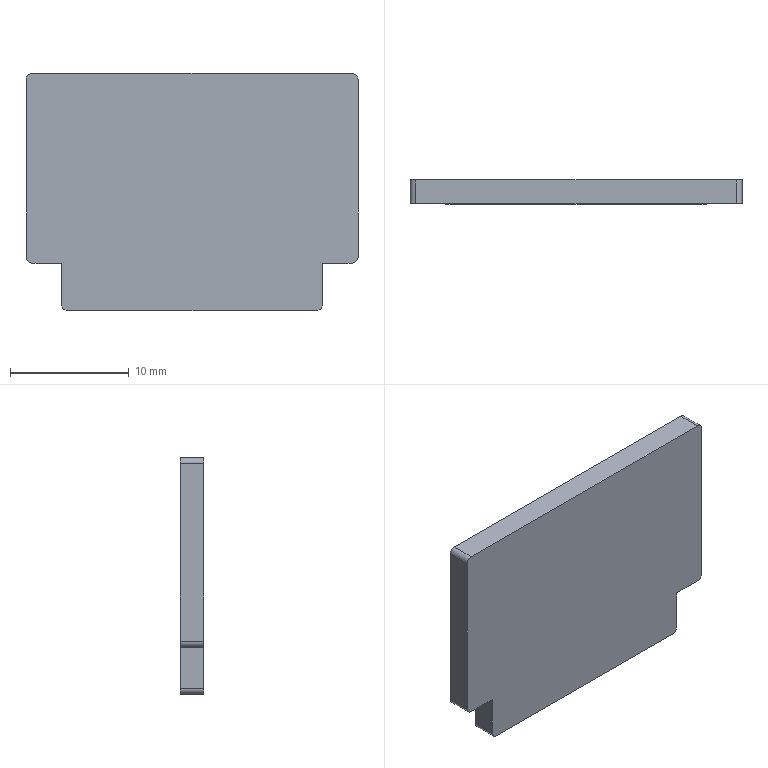Part | STEP file | Second C-100-B Work Part | 1 solid | 16 faces | box 28 x 2 x 20 mm | volume 1071 mm3 | plane 10 | cylinder 6 | commonest cylinder face diameters 1 x6
STEP:
#1=CARTESIAN_POINT('',(-11.,2.,-14.2));
#2=VERTEX_POINT('',#1);
#3=CARTESIAN_POINT('',(-10.5,2.,-14.7));
#4=VERTEX_POINT('',#3);
#5=CARTESIAN_POINT('',(-10.5,2.,-14.2));
#6=DIRECTION('',(0.,-1.,0.));
#7=DIRECTION('',(0.,0.,-1.));
#8=AXIS2_PLACEMENT_3D('',#5,#6,#7);
#9=CIRCLE('',#8,0.5);
#10=EDGE_CURVE('',#2,#4,#9,.T.);
#11=ORIENTED_EDGE('',*,*,#10,.F.);
#12=CARTESIAN_POINT('',(-11.,2.,-10.7));
#13=VERTEX_POINT('',#12);
#14=CARTESIAN_POINT('',(-11.,2.,-10.2));
#15=DIRECTION('',(0.,0.,1.));
#16=VECTOR('',#15,1000.);
#17=LINE('',#14,#16);
#18=EDGE_CURVE('',#2,#13,#17,.T.);
#19=ORIENTED_EDGE('',*,*,#18,.T.);
#20=CARTESIAN_POINT('',(-13.5,2.,-10.7));
#21=VERTEX_POINT('',#20);
#22=CARTESIAN_POINT('',(-13.5,2.,-10.7));
#23=DIRECTION('',(-1.,0.,0.));
#24=VECTOR('',#23,1000.);
#25=LINE('',#22,#24);
#26=EDGE_CURVE('',#13,#21,#25,.T.);
#27=ORIENTED_EDGE('',*,*,#26,.T.);
#28=CARTESIAN_POINT('',(-14.,2.,-10.2));
#29=VERTEX_POINT('',#28);
#30=CARTESIAN_POINT('',(-13.5,2.,-10.2));
#31=DIRECTION('',(0.,-1.,0.));
#32=DIRECTION('',(0.,0.,-1.));
#33=AXIS2_PLACEMENT_3D('',#30,#31,#32);
#34=CIRCLE('',#33,0.5);
#35=EDGE_CURVE('',#29,#21,#34,.T.);
#36=ORIENTED_EDGE('',*,*,#35,.F.);
#37=CARTESIAN_POINT('',(-14.,2.,4.8));
#38=VERTEX_POINT('',#37);
#39=CARTESIAN_POINT('',(-14.,2.,-10.2));
#40=DIRECTION('',(0.,0.,1.));
#41=VECTOR('',#40,1000.);
#42=LINE('',#39,#41);
#43=EDGE_CURVE('',#29,#38,#42,.T.);
#44=ORIENTED_EDGE('',*,*,#43,.T.);
#45=CARTESIAN_POINT('',(-13.5,2.,5.3));
#46=VERTEX_POINT('',#45);
#47=CARTESIAN_POINT('',(-13.5,2.,4.8));
#48=DIRECTION('',(0.,-1.,0.));
#49=DIRECTION('',(0.,0.,-1.));
#50=AXIS2_PLACEMENT_3D('',#47,#48,#49);
#51=CIRCLE('',#50,0.5);
#52=EDGE_CURVE('',#46,#38,#51,.T.);
#53=ORIENTED_EDGE('',*,*,#52,.F.);
#54=CARTESIAN_POINT('',(13.5,2.,5.3));
#55=VERTEX_POINT('',#54);
#56=CARTESIAN_POINT('',(-13.5,2.,5.3));
#57=DIRECTION('',(1.,0.,0.));
#58=VECTOR('',#57,1000.);
#59=LINE('',#56,#58);
#60=EDGE_CURVE('',#46,#55,#59,.T.);
#61=ORIENTED_EDGE('',*,*,#60,.T.);
#62=CARTESIAN_POINT('',(14.,2.,4.8));
#63=VERTEX_POINT('',#62);
#64=CARTESIAN_POINT('',(13.5,2.,4.8));
#65=DIRECTION('',(0.,-1.,0.));
#66=DIRECTION('',(0.,0.,-1.));
#67=AXIS2_PLACEMENT_3D('',#64,#65,#66);
#68=CIRCLE('',#67,0.5);
#69=EDGE_CURVE('',#63,#55,#68,.T.);
#70=ORIENTED_EDGE('',*,*,#69,.F.);
#71=CARTESIAN_POINT('',(14.,2.,-10.2));
#72=VERTEX_POINT('',#71);
#73=CARTESIAN_POINT('',(14.,2.,-10.2));
#74=DIRECTION('',(0.,0.,-1.));
#75=VECTOR('',#74,1000.);
#76=LINE('',#73,#75);
#77=EDGE_CURVE('',#63,#72,#76,.T.);
#78=ORIENTED_EDGE('',*,*,#77,.T.);
#79=CARTESIAN_POINT('',(13.5,2.,-10.7));
#80=VERTEX_POINT('',#79);
#81=CARTESIAN_POINT('',(13.5,2.,-10.2));
#82=DIRECTION('',(0.,-1.,0.));
#83=DIRECTION('',(0.,0.,-1.));
#84=AXIS2_PLACEMENT_3D('',#81,#82,#83);
#85=CIRCLE('',#84,0.5);
#86=EDGE_CURVE('',#80,#72,#85,.T.);
#87=ORIENTED_EDGE('',*,*,#86,.F.);
#88=CARTESIAN_POINT('',(11.,2.,-10.7));
#89=VERTEX_POINT('',#88);
#90=CARTESIAN_POINT('',(-13.5,2.,-10.7));
#91=DIRECTION('',(-1.,0.,0.));
#92=VECTOR('',#91,1000.);
#93=LINE('',#90,#92);
#94=EDGE_CURVE('',#80,#89,#93,.T.);
#95=ORIENTED_EDGE('',*,*,#94,.T.);
#96=CARTESIAN_POINT('',(11.,2.,-14.2));
#97=VERTEX_POINT('',#96);
#98=CARTESIAN_POINT('',(11.,2.,-10.2));
#99=DIRECTION('',(0.,0.,-1.));
#100=VECTOR('',#99,1000.);
#101=LINE('',#98,#100);
#102=EDGE_CURVE('',#89,#97,#101,.T.);
#103=ORIENTED_EDGE('',*,*,#102,.T.);
#104=CARTESIAN_POINT('',(10.5,2.,-14.7));
#105=VERTEX_POINT('',#104);
#106=CARTESIAN_POINT('',(10.5,2.,-14.2));
#107=DIRECTION('',(0.,-1.,0.));
#108=DIRECTION('',(0.,0.,-1.));
#109=AXIS2_PLACEMENT_3D('',#106,#107,#108);
#110=CIRCLE('',#109,0.5);
#111=EDGE_CURVE('',#105,#97,#110,.T.);
#112=ORIENTED_EDGE('',*,*,#111,.F.);
#113=CARTESIAN_POINT('',(-13.5,2.,-14.7));
#114=DIRECTION('',(-1.,0.,0.));
#115=VECTOR('',#114,1000.);
#116=LINE('',#113,#115);
#117=EDGE_CURVE('',#105,#4,#116,.T.);
#118=ORIENTED_EDGE('',*,*,#117,.T.);
#119=EDGE_LOOP('',(#11,#19,#27,#36,#44,#53,#61,#70,#78,#87,#95,#103,#112,#118));
#120=FACE_OUTER_BOUND('',#119,.T.);
#121=CARTESIAN_POINT('',(-13.5,2.,-10.2));
#122=DIRECTION('',(0.,1.,0.));
#123=DIRECTION('',(0.,0.,1.));
#124=AXIS2_PLACEMENT_3D('',#121,#122,#123);
#125=PLANE('',#124);
#126=ADVANCED_FACE('',(#120),#125,.T.);
#127=CARTESIAN_POINT('',(-11.,0.,-10.7));
#128=VERTEX_POINT('',#127);
#129=CARTESIAN_POINT('',(-11.,2.,-10.7));
#130=DIRECTION('',(0.,-1.,0.));
#131=VECTOR('',#130,1000.);
#132=LINE('',#129,#131);
#133=EDGE_CURVE('',#13,#128,#132,.T.);
#134=ORIENTED_EDGE('',*,*,#133,.F.);
#135=ORIENTED_EDGE('',*,*,#18,.F.);
#136=CARTESIAN_POINT('',(-11.,0.,-14.2));
#137=VERTEX_POINT('',#136);
#138=CARTESIAN_POINT('',(-11.,2.,-14.2));
#139=DIRECTION('',(0.,1.,0.));
#140=VECTOR('',#139,1000.);
#141=LINE('',#138,#140);
#142=EDGE_CURVE('',#137,#2,#141,.T.);
#143=ORIENTED_EDGE('',*,*,#142,.F.);
#144=CARTESIAN_POINT('',(-11.,0.,-10.7));
#145=DIRECTION('',(0.,0.,-1.));
#146=VECTOR('',#145,1000.);
#147=LINE('',#144,#146);
#148=EDGE_CURVE('',#128,#137,#147,.T.);
#149=ORIENTED_EDGE('',*,*,#148,.F.);
#150=EDGE_LOOP('',(#134,#135,#143,#149));
#151=FACE_OUTER_BOUND('',#150,.T.);
#152=CARTESIAN_POINT('',(-11.,2.,-10.7));
#153=DIRECTION('',(1.,0.,0.));
#154=DIRECTION('',(0.,0.,-1.));
#155=AXIS2_PLACEMENT_3D('',#152,#153,#154);
#156=PLANE('',#155);
#157=ADVANCED_FACE('',(#151),#156,.F.);
#158=CARTESIAN_POINT('',(-10.5,0.,-14.7));
#159=VERTEX_POINT('',#158);
#160=CARTESIAN_POINT('',(-10.5,2.,-14.7));
#161=DIRECTION('',(0.,-1.,0.));
#162=VECTOR('',#161,1000.);
#163=LINE('',#160,#162);
#164=EDGE_CURVE('',#4,#159,#163,.T.);
#165=ORIENTED_EDGE('',*,*,#164,.F.);
#166=ORIENTED_EDGE('',*,*,#117,.F.);
#167=CARTESIAN_POINT('',(10.5,0.,-14.7));
#168=VERTEX_POINT('',#167);
#169=CARTESIAN_POINT('',(10.5,2.,-14.7));
#170=DIRECTION('',(0.,1.,0.));
#171=VECTOR('',#170,1000.);
#172=LINE('',#169,#171);
#173=EDGE_CURVE('',#168,#105,#172,.T.);
#174=ORIENTED_EDGE('',*,*,#173,.F.);
#175=CARTESIAN_POINT('',(-10.5,0.,-14.7));
#176=DIRECTION('',(1.,0.,0.));
#177=VECTOR('',#176,1000.);
#178=LINE('',#175,#177);
#179=EDGE_CURVE('',#159,#168,#178,.T.);
#180=ORIENTED_EDGE('',*,*,#179,.F.);
#181=EDGE_LOOP('',(#165,#166,#174,#180));
#182=FACE_OUTER_BOUND('',#181,.T.);
#183=CARTESIAN_POINT('',(-10.5,2.,-14.7));
#184=DIRECTION('',(0.,0.,1.));
#185=DIRECTION('',(1.,0.,0.));
#186=AXIS2_PLACEMENT_3D('',#183,#184,#185);
#187=PLANE('',#186);
#188=ADVANCED_FACE('',(#182),#187,.F.);
#189=CARTESIAN_POINT('',(11.,0.,-14.2));
#190=VERTEX_POINT('',#189);
#191=CARTESIAN_POINT('',(11.,2.,-14.2));
#192=DIRECTION('',(0.,-1.,0.));
#193=VECTOR('',#192,1000.);
#194=LINE('',#191,#193);
#195=EDGE_CURVE('',#97,#190,#194,.T.);
#196=ORIENTED_EDGE('',*,*,#195,.F.);
#197=ORIENTED_EDGE('',*,*,#102,.F.);
#198=CARTESIAN_POINT('',(11.,0.,-10.7));
#199=VERTEX_POINT('',#198);
#200=CARTESIAN_POINT('',(11.,2.,-10.7));
#201=DIRECTION('',(0.,1.,0.));
#202=VECTOR('',#201,1000.);
#203=LINE('',#200,#202);
#204=EDGE_CURVE('',#199,#89,#203,.T.);
#205=ORIENTED_EDGE('',*,*,#204,.F.);
#206=CARTESIAN_POINT('',(11.,0.,-14.2));
#207=DIRECTION('',(0.,0.,1.));
#208=VECTOR('',#207,1000.);
#209=LINE('',#206,#208);
#210=EDGE_CURVE('',#190,#199,#209,.T.);
#211=ORIENTED_EDGE('',*,*,#210,.F.);
#212=EDGE_LOOP('',(#196,#197,#205,#211));
#213=FACE_OUTER_BOUND('',#212,.T.);
#214=CARTESIAN_POINT('',(11.,2.,-14.2));
#215=DIRECTION('',(-1.,0.,0.));
#216=DIRECTION('',(0.,0.,1.));
#217=AXIS2_PLACEMENT_3D('',#214,#215,#216);
#218=PLANE('',#217);
#219=ADVANCED_FACE('',(#213),#218,.F.);
#220=ORIENTED_EDGE('',*,*,#204,.T.);
#221=ORIENTED_EDGE('',*,*,#94,.F.);
#222=CARTESIAN_POINT('',(13.5,0.,-10.7));
#223=VERTEX_POINT('',#222);
#224=CARTESIAN_POINT('',(13.5,2.,-10.7));
#225=DIRECTION('',(0.,1.,0.));
#226=VECTOR('',#225,1000.);
#227=LINE('',#224,#226);
#228=EDGE_CURVE('',#223,#80,#227,.T.);
#229=ORIENTED_EDGE('',*,*,#228,.F.);
#230=CARTESIAN_POINT('',(13.5,0.,-10.7));
#231=DIRECTION('',(1.,0.,0.));
#232=VECTOR('',#231,1000.);
#233=LINE('',#230,#232);
#234=EDGE_CURVE('',#199,#223,#233,.T.);
#235=ORIENTED_EDGE('',*,*,#234,.F.);
#236=EDGE_LOOP('',(#220,#221,#229,#235));
#237=FACE_OUTER_BOUND('',#236,.T.);
#238=CARTESIAN_POINT('',(13.5,2.,-10.7));
#239=DIRECTION('',(0.,0.,1.));
#240=DIRECTION('',(1.,0.,0.));
#241=AXIS2_PLACEMENT_3D('',#238,#239,#240);
#242=PLANE('',#241);
#243=ADVANCED_FACE('',(#237),#242,.F.);
#244=CARTESIAN_POINT('',(14.,0.,-10.2));
#245=VERTEX_POINT('',#244);
#246=CARTESIAN_POINT('',(14.,2.,-10.2));
#247=DIRECTION('',(0.,-1.,0.));
#248=VECTOR('',#247,1000.);
#249=LINE('',#246,#248);
#250=EDGE_CURVE('',#72,#245,#249,.T.);
#251=ORIENTED_EDGE('',*,*,#250,.F.);
#252=ORIENTED_EDGE('',*,*,#77,.F.);
#253=CARTESIAN_POINT('',(14.,0.,4.8));
#254=VERTEX_POINT('',#253);
#255=CARTESIAN_POINT('',(14.,2.,4.8));
#256=DIRECTION('',(0.,1.,0.));
#257=VECTOR('',#256,1000.);
#258=LINE('',#255,#257);
#259=EDGE_CURVE('',#254,#63,#258,.T.);
#260=ORIENTED_EDGE('',*,*,#259,.F.);
#261=CARTESIAN_POINT('',(14.,0.,4.8));
#262=DIRECTION('',(0.,0.,1.));
#263=VECTOR('',#262,1000.);
#264=LINE('',#261,#263);
#265=EDGE_CURVE('',#245,#254,#264,.T.);
#266=ORIENTED_EDGE('',*,*,#265,.F.);
#267=EDGE_LOOP('',(#251,#252,#260,#266));
#268=FACE_OUTER_BOUND('',#267,.T.);
#269=CARTESIAN_POINT('',(14.,2.,4.8));
#270=DIRECTION('',(-1.,0.,0.));
#271=DIRECTION('',(0.,0.,1.));
#272=AXIS2_PLACEMENT_3D('',#269,#270,#271);
#273=PLANE('',#272);
#274=ADVANCED_FACE('',(#268),#273,.F.);
#275=CARTESIAN_POINT('',(13.5,0.,5.3));
#276=VERTEX_POINT('',#275);
#277=CARTESIAN_POINT('',(13.5,2.,5.3));
#278=DIRECTION('',(0.,-1.,0.));
#279=VECTOR('',#278,1000.);
#280=LINE('',#277,#279);
#281=EDGE_CURVE('',#55,#276,#280,.T.);
#282=ORIENTED_EDGE('',*,*,#281,.F.);
#283=ORIENTED_EDGE('',*,*,#60,.F.);
#284=CARTESIAN_POINT('',(-13.5,0.,5.3));
#285=VERTEX_POINT('',#284);
#286=CARTESIAN_POINT('',(-13.5,2.,5.3));
#287=DIRECTION('',(0.,1.,0.));
#288=VECTOR('',#287,1000.);
#289=LINE('',#286,#288);
#290=EDGE_CURVE('',#285,#46,#289,.T.);
#291=ORIENTED_EDGE('',*,*,#290,.F.);
#292=CARTESIAN_POINT('',(-13.5,0.,5.3));
#293=DIRECTION('',(-1.,0.,0.));
#294=VECTOR('',#293,1000.);
#295=LINE('',#292,#294);
#296=EDGE_CURVE('',#276,#285,#295,.T.);
#297=ORIENTED_EDGE('',*,*,#296,.F.);
#298=EDGE_LOOP('',(#282,#283,#291,#297));
#299=FACE_OUTER_BOUND('',#298,.T.);
#300=CARTESIAN_POINT('',(-13.5,2.,5.3));
#301=DIRECTION('',(0.,0.,-1.));
#302=DIRECTION('',(-1.,0.,0.));
#303=AXIS2_PLACEMENT_3D('',#300,#301,#302);
#304=PLANE('',#303);
#305=ADVANCED_FACE('',(#299),#304,.F.);
#306=CARTESIAN_POINT('',(-14.,0.,4.8));
#307=VERTEX_POINT('',#306);
#308=CARTESIAN_POINT('',(-14.,2.,4.8));
#309=DIRECTION('',(0.,-1.,0.));
#310=VECTOR('',#309,1000.);
#311=LINE('',#308,#310);
#312=EDGE_CURVE('',#38,#307,#311,.T.);
#313=ORIENTED_EDGE('',*,*,#312,.F.);
#314=ORIENTED_EDGE('',*,*,#43,.F.);
#315=CARTESIAN_POINT('',(-14.,0.,-10.2));
#316=VERTEX_POINT('',#315);
#317=CARTESIAN_POINT('',(-14.,2.,-10.2));
#318=DIRECTION('',(0.,1.,0.));
#319=VECTOR('',#318,1000.);
#320=LINE('',#317,#319);
#321=EDGE_CURVE('',#316,#29,#320,.T.);
#322=ORIENTED_EDGE('',*,*,#321,.F.);
#323=CARTESIAN_POINT('',(-14.,0.,-10.2));
#324=DIRECTION('',(0.,0.,-1.));
#325=VECTOR('',#324,1000.);
#326=LINE('',#323,#325);
#327=EDGE_CURVE('',#307,#316,#326,.T.);
#328=ORIENTED_EDGE('',*,*,#327,.F.);
#329=EDGE_LOOP('',(#313,#314,#322,#328));
#330=FACE_OUTER_BOUND('',#329,.T.);
#331=CARTESIAN_POINT('',(-14.,2.,-10.2));
#332=DIRECTION('',(1.,0.,0.));
#333=DIRECTION('',(0.,0.,-1.));
#334=AXIS2_PLACEMENT_3D('',#331,#332,#333);
#335=PLANE('',#334);
#336=ADVANCED_FACE('',(#330),#335,.F.);
#337=CARTESIAN_POINT('',(-13.5,0.,-10.7));
#338=VERTEX_POINT('',#337);
#339=CARTESIAN_POINT('',(-13.5,2.,-10.7));
#340=DIRECTION('',(0.,-1.,0.));
#341=VECTOR('',#340,1000.);
#342=LINE('',#339,#341);
#343=EDGE_CURVE('',#21,#338,#342,.T.);
#344=ORIENTED_EDGE('',*,*,#343,.F.);
#345=ORIENTED_EDGE('',*,*,#26,.F.);
#346=ORIENTED_EDGE('',*,*,#133,.T.);
#347=CARTESIAN_POINT('',(-11.,0.,-10.7));
#348=DIRECTION('',(1.,0.,0.));
#349=VECTOR('',#348,1000.);
#350=LINE('',#347,#349);
#351=EDGE_CURVE('',#338,#128,#350,.T.);
#352=ORIENTED_EDGE('',*,*,#351,.F.);
#353=EDGE_LOOP('',(#344,#345,#346,#352));
#354=FACE_OUTER_BOUND('',#353,.T.);
#355=CARTESIAN_POINT('',(-11.,2.,-10.7));
#356=DIRECTION('',(0.,0.,1.));
#357=DIRECTION('',(1.,0.,0.));
#358=AXIS2_PLACEMENT_3D('',#355,#356,#357);
#359=PLANE('',#358);
#360=ADVANCED_FACE('',(#354),#359,.F.);
#361=ORIENTED_EDGE('',*,*,#148,.T.);
#362=CARTESIAN_POINT('',(-10.5,0.,-14.2));
#363=DIRECTION('',(0.,1.,0.));
#364=DIRECTION('',(0.,0.,-1.));
#365=AXIS2_PLACEMENT_3D('',#362,#363,#364);
#366=CIRCLE('',#365,0.5);
#367=EDGE_CURVE('',#159,#137,#366,.T.);
#368=ORIENTED_EDGE('',*,*,#367,.F.);
#369=ORIENTED_EDGE('',*,*,#179,.T.);
#370=CARTESIAN_POINT('',(10.5,0.,-14.2));
#371=DIRECTION('',(0.,1.,0.));
#372=DIRECTION('',(0.,0.,-1.));
#373=AXIS2_PLACEMENT_3D('',#370,#371,#372);
#374=CIRCLE('',#373,0.5);
#375=EDGE_CURVE('',#190,#168,#374,.T.);
#376=ORIENTED_EDGE('',*,*,#375,.F.);
#377=ORIENTED_EDGE('',*,*,#210,.T.);
#378=ORIENTED_EDGE('',*,*,#234,.T.);
#379=CARTESIAN_POINT('',(13.5,0.,-10.2));
#380=DIRECTION('',(0.,1.,0.));
#381=DIRECTION('',(0.,0.,-1.));
#382=AXIS2_PLACEMENT_3D('',#379,#380,#381);
#383=CIRCLE('',#382,0.5);
#384=EDGE_CURVE('',#245,#223,#383,.T.);
#385=ORIENTED_EDGE('',*,*,#384,.F.);
#386=ORIENTED_EDGE('',*,*,#265,.T.);
#387=CARTESIAN_POINT('',(13.5,0.,4.8));
#388=DIRECTION('',(0.,1.,0.));
#389=DIRECTION('',(0.,0.,-1.));
#390=AXIS2_PLACEMENT_3D('',#387,#388,#389);
#391=CIRCLE('',#390,0.5);
#392=EDGE_CURVE('',#276,#254,#391,.T.);
#393=ORIENTED_EDGE('',*,*,#392,.F.);
#394=ORIENTED_EDGE('',*,*,#296,.T.);
#395=CARTESIAN_POINT('',(-13.5,0.,4.8));
#396=DIRECTION('',(0.,1.,0.));
#397=DIRECTION('',(0.,0.,-1.));
#398=AXIS2_PLACEMENT_3D('',#395,#396,#397);
#399=CIRCLE('',#398,0.5);
#400=EDGE_CURVE('',#307,#285,#399,.T.);
#401=ORIENTED_EDGE('',*,*,#400,.F.);
#402=ORIENTED_EDGE('',*,*,#327,.T.);
#403=CARTESIAN_POINT('',(-13.5,0.,-10.2));
#404=DIRECTION('',(0.,1.,0.));
#405=DIRECTION('',(0.,0.,-1.));
#406=AXIS2_PLACEMENT_3D('',#403,#404,#405);
#407=CIRCLE('',#406,0.5);
#408=EDGE_CURVE('',#338,#316,#407,.T.);
#409=ORIENTED_EDGE('',*,*,#408,.F.);
#410=ORIENTED_EDGE('',*,*,#351,.T.);
#411=EDGE_LOOP('',(#361,#368,#369,#376,#377,#378,#385,#386,#393,#394,#401,#402,#409,#410));
#412=FACE_OUTER_BOUND('',#411,.T.);
#413=CARTESIAN_POINT('',(-13.5,0.,-10.2));
#414=DIRECTION('',(0.,1.,0.));
#415=DIRECTION('',(0.,0.,1.));
#416=AXIS2_PLACEMENT_3D('',#413,#414,#415);
#417=PLANE('',#416);
#418=ADVANCED_FACE('',(#412),#417,.F.);
#419=ORIENTED_EDGE('',*,*,#10,.T.);
#420=ORIENTED_EDGE('',*,*,#164,.T.);
#421=ORIENTED_EDGE('',*,*,#367,.T.);
#422=ORIENTED_EDGE('',*,*,#142,.T.);
#423=EDGE_LOOP('',(#419,#420,#421,#422));
#424=FACE_OUTER_BOUND('',#423,.T.);
#425=CARTESIAN_POINT('',(-10.5,2.,-14.2));
#426=DIRECTION('',(0.,-1.,0.));
#427=DIRECTION('',(0.,0.,-1.));
#428=AXIS2_PLACEMENT_3D('',#425,#426,#427);
#429=CYLINDRICAL_SURFACE('',#428,0.5);
#430=ADVANCED_FACE('',(#424),#429,.T.);
#431=ORIENTED_EDGE('',*,*,#111,.T.);
#432=ORIENTED_EDGE('',*,*,#195,.T.);
#433=ORIENTED_EDGE('',*,*,#375,.T.);
#434=ORIENTED_EDGE('',*,*,#173,.T.);
#435=EDGE_LOOP('',(#431,#432,#433,#434));
#436=FACE_OUTER_BOUND('',#435,.T.);
#437=CARTESIAN_POINT('',(10.5,2.,-14.2));
#438=DIRECTION('',(0.,-1.,0.));
#439=DIRECTION('',(0.,0.,-1.));
#440=AXIS2_PLACEMENT_3D('',#437,#438,#439);
#441=CYLINDRICAL_SURFACE('',#440,0.5);
#442=ADVANCED_FACE('',(#436),#441,.T.);
#443=ORIENTED_EDGE('',*,*,#86,.T.);
#444=ORIENTED_EDGE('',*,*,#250,.T.);
#445=ORIENTED_EDGE('',*,*,#384,.T.);
#446=ORIENTED_EDGE('',*,*,#228,.T.);
#447=EDGE_LOOP('',(#443,#444,#445,#446));
#448=FACE_OUTER_BOUND('',#447,.T.);
#449=CARTESIAN_POINT('',(13.5,2.,-10.2));
#450=DIRECTION('',(0.,-1.,0.));
#451=DIRECTION('',(0.,0.,-1.));
#452=AXIS2_PLACEMENT_3D('',#449,#450,#451);
#453=CYLINDRICAL_SURFACE('',#452,0.5);
#454=ADVANCED_FACE('',(#448),#453,.T.);
#455=ORIENTED_EDGE('',*,*,#69,.T.);
#456=ORIENTED_EDGE('',*,*,#281,.T.);
#457=ORIENTED_EDGE('',*,*,#392,.T.);
#458=ORIENTED_EDGE('',*,*,#259,.T.);
#459=EDGE_LOOP('',(#455,#456,#457,#458));
#460=FACE_OUTER_BOUND('',#459,.T.);
#461=CARTESIAN_POINT('',(13.5,2.,4.8));
#462=DIRECTION('',(0.,-1.,0.));
#463=DIRECTION('',(0.,0.,-1.));
#464=AXIS2_PLACEMENT_3D('',#461,#462,#463);
#465=CYLINDRICAL_SURFACE('',#464,0.5);
#466=ADVANCED_FACE('',(#460),#465,.T.);
#467=ORIENTED_EDGE('',*,*,#52,.T.);
#468=ORIENTED_EDGE('',*,*,#312,.T.);
#469=ORIENTED_EDGE('',*,*,#400,.T.);
#470=ORIENTED_EDGE('',*,*,#290,.T.);
#471=EDGE_LOOP('',(#467,#468,#469,#470));
#472=FACE_OUTER_BOUND('',#471,.T.);
#473=CARTESIAN_POINT('',(-13.5,2.,4.8));
#474=DIRECTION('',(0.,-1.,0.));
#475=DIRECTION('',(0.,0.,-1.));
#476=AXIS2_PLACEMENT_3D('',#473,#474,#475);
#477=CYLINDRICAL_SURFACE('',#476,0.5);
#478=ADVANCED_FACE('',(#472),#477,.T.);
#479=ORIENTED_EDGE('',*,*,#35,.T.);
#480=ORIENTED_EDGE('',*,*,#343,.T.);
#481=ORIENTED_EDGE('',*,*,#408,.T.);
#482=ORIENTED_EDGE('',*,*,#321,.T.);
#483=EDGE_LOOP('',(#479,#480,#481,#482));
#484=FACE_OUTER_BOUND('',#483,.T.);
#485=CARTESIAN_POINT('',(-13.5,2.,-10.2));
#486=DIRECTION('',(0.,-1.,0.));
#487=DIRECTION('',(0.,0.,-1.));
#488=AXIS2_PLACEMENT_3D('',#485,#486,#487);
#489=CYLINDRICAL_SURFACE('',#488,0.5);
#490=ADVANCED_FACE('',(#484),#489,.T.);
#491=CLOSED_SHELL('',(#126,#157,#188,#219,#243,#274,#305,#336,#360,#418,#430,#442,#454,#466,#478,#490));
#492=MANIFOLD_SOLID_BREP('',#491);
#493=CARTESIAN_POINT('',(0.,0.,0.));
#494=DIRECTION('',(0.,0.,1.));
#495=DIRECTION('',(1.,0.,0.));
#496=AXIS2_PLACEMENT_3D('',#493,#494,#495);
#497=(LENGTH_UNIT()NAMED_UNIT(*)SI_UNIT(.MILLI.,.METRE.));
#498=UNCERTAINTY_MEASURE_WITH_UNIT(LENGTH_MEASURE(0.00001),#497,'','');
#499=(NAMED_UNIT(*)PLANE_ANGLE_UNIT()SI_UNIT($,.RADIAN.));
#500=(NAMED_UNIT(*)SI_UNIT($,.STERADIAN.)SOLID_ANGLE_UNIT());
#501=(GEOMETRIC_REPRESENTATION_CONTEXT(3)GLOBAL_UNCERTAINTY_ASSIGNED_CONTEXT((#498))GLOBAL_UNIT_ASSIGNED_CONTEXT((#497,#499,#500))REPRESENTATION_CONTEXT('',''));
#502=ADVANCED_BREP_SHAPE_REPRESENTATION('',(#492,#496),#501);